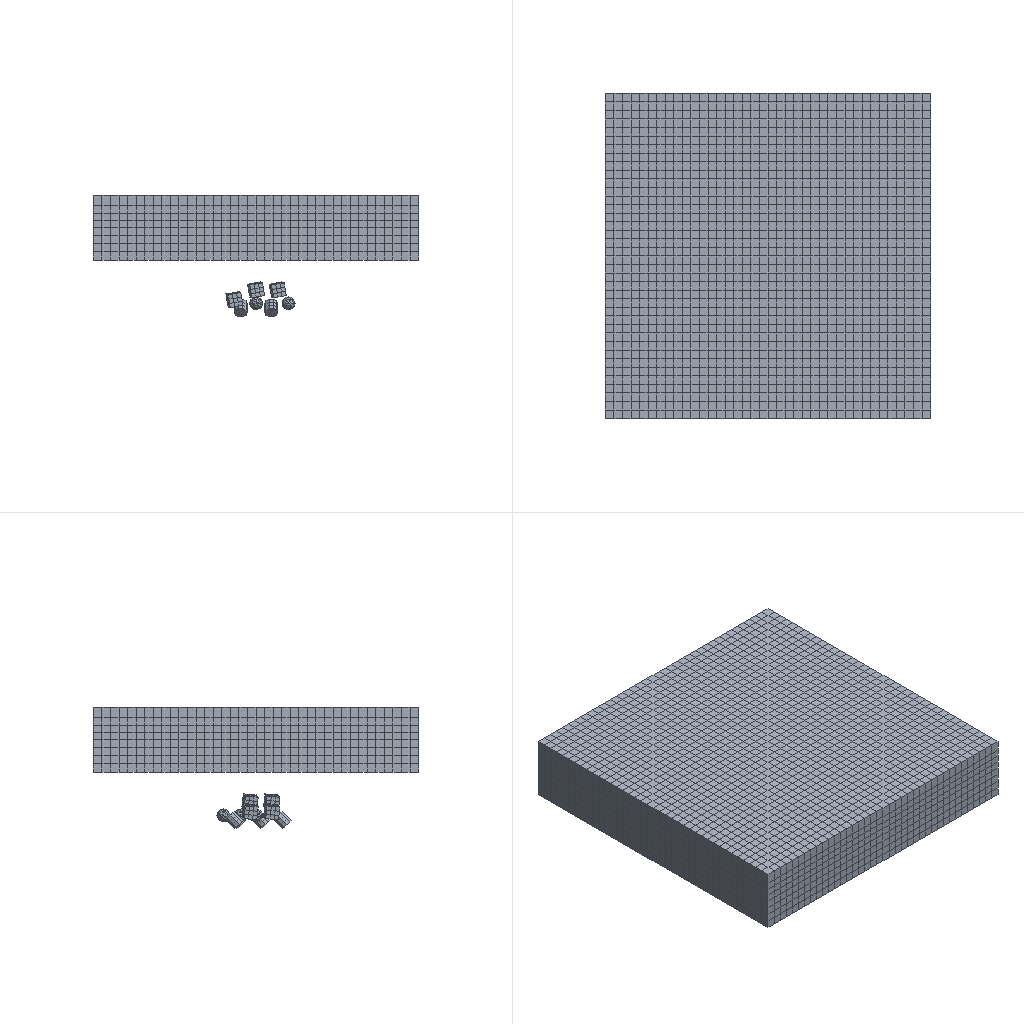Simulation study | abaqus
Set-up summary:
category,name,step,type,value,unit,region
solver,abaqus
solver,version,,,Abaqus/Standard 2020
units,not stated in the deck,,not stated
analysis,deck,,transient,transient
load_step,Step-1,Step-1,transient
load_step,requested,,,1
mesh,nodes,,,19847
mesh,elements,,,15155
element_type,C3D8R,,solid,11870
element_type,C3D10M,,solid,3285
load,load commands in deck,,count,1
bc,support commands in deck,,count,1
material,NIANTU,,in results
material,SHATU,,in results
material,SHI,,in results
material,YUNI,,in results
check,setup vs results,,match,"per instance, exact: element labels, types and connectivity; labels of the nodes the elements use; coordinates of those nodes at SINGLE_PRECISION in 15 of 16 instance(s)"
Abaqus input file, long lists of numbers shortened:
*Heading
** Job name: Job-2 Model name: Model-1-Copy
** Generated by: Abaqus/CAE 2020
*Preprint, echo=NO, model=NO, history=NO, contact=NO
**
** PARTS
**
*Part, name=base
*Node
      1,           0.,           0.,          1.5
      2,           0.,         -15.,          1.5
** (13687 more lines like these left out)
*Element, type=C3D8R
   1,  246,  925, 6845,  777,    1,   17,  629,   94
   2,  925,  926, 6846, 6845,   17,   18,  630,  629
** (11550 more lines like these left out)
*Nset, nset=Set-1
    3,    4,    6,    7,   13,   14,   15,   16,   56,   57,   58,   59,   60,   61,   62,   63
   64,   65,   66,   67,   68,   69,   70,   71,   72,   73,   74,   75,   76,   77,   78,   79
** (189 more lines like these left out)
*Elset, elset=Set-1, generate
 10109,  11552,      1
*Nset, nset=Set-2
    1,    2,    3,    4,    5,    6,    7,    8,   17,   18,   19,   20,   21,   22,   23,   24
   25,   26,   27,   28,   29,   30,   31,   32,   33,   34,   35,   36,   37,   38,   39,   40
** (379 more lines like these left out)
*Elset, elset=Set-2, generate
    1,  4332,     1
*Nset, nset=Set-3
     1,     2,     5,     8,     9,    10,    11,    12,    17,    18,    19,    20,    21,    22,    23,    24
    25,    26,    27,    28,    29,    30,    31,    32,    33,    34,    35,    36,    37,    38,    39,    40
** (474 more lines like these left out)
*Elset, elset=Set-3, generate
  4333,  10108,      1
** Section: niantu
*Solid Section, elset=Set-2, material=niantu
,
** Section: shatu
*Solid Section, elset=Set-3, material=shatu
,
** Section: yuni
*Solid Section, elset=Set-1, material=yuni
,
*End Part
**
*Part, name=fang
*Node
      1,           0., -0.6,  0.6
      2,           0., -0.4,  0.6
** (62 more lines like these left out)
*Element, type=C3D8R
 1, 17, 18, 22, 21,  1,  2,  6,  5
 2, 18, 19, 23, 22,  2,  3,  7,  6
** (25 more lines like these left out)
*Nset, nset=Set-1, generate
  1,  64,   1
*Elset, elset=Set-1, generate
  1,  27,   1
** Section: shi
*Solid Section, elset=Set-1, material=shi
,
*End Part
**
*Part, name=fangkuai
*Node
      1,  0.2427,           0.,  0.1763
      2, 0.09271,           0.,  0.2853
** (74 more lines like these left out)
*Element, type=C3D8R
 1,  6,  7,  8, 19, 25, 26, 27, 38
 2, 11, 14, 12, 19, 30, 33, 31, 38
** (37 more lines like these left out)
*Nset, nset=Set-1, generate
  1,  76,   1
*Elset, elset=Set-1, generate
  1,  39,   1
** Section: shi
*Solid Section, elset=Set-1, material=shi
,
*End Part
**
*Part, name=sphere
*Node
      1,  0.1148,  0.2772,           0.
      2,  0.2121,  0.2121,           0.
** (1092 more lines like these left out)
*Element, type=C3D10M
  1,  101,  102,  103,  104,  173,  172,  171,  175,  174,  176
  2,  105,  106,  102,  107,  179,  178,  177,  181,  180,  182
** (655 more lines like these left out)
*Nset, nset=Set-1, generate
    1,  1094,     1
*Elset, elset=Set-1, generate
   1,  657,    1
** Section: shi
*Solid Section, elset=Set-1, material=shi
,
*End Part
**
**
** ASSEMBLY
**
*Assembly, name=Assembly
**
*Instance, name=base-1, part=base
*End Instance
**
*Instance, name=sphere-1, part=sphere
         7.5,         -7.5,          -2.
*End Instance
**
*Instance, name=fangkuai-1, part=fangkuai
         8.2,         -7.5,          -2.
         8.2,         -7.5,          -2., 9.2,         -7.5,          -2., 45.
*End Instance
**
*Instance, name=fang-1, part=fang
6.209, -6.949, -2.154
6.209, -6.949, -2.154, 6.542, -7.616, -1.487, 15.
*End Instance
**
*Instance, name=sphere-1-lin-1-2, part=sphere
         7.5,         -6.8,          -2.
*End Instance
**
*Instance, name=sphere-1-lin-2-1, part=sphere
          9.,         -7.5,          -2.
*End Instance
**
*Instance, name=sphere-1-lin-2-2, part=sphere
          9.,         -6.8,          -2.
*End Instance
**
*Instance, name=fangkuai-1-lin-1-2, part=fangkuai
         8.2,         -6.4,          -2.
         8.2,         -6.4,          -2., 9.2,         -6.4,          -2., 45.
*End Instance
**
*Instance, name=fangkuai-1-lin-1-2-1, part=fangkuai
         8.2,         -8.5,          -2.
         8.2,         -8.5,          -2., 9.2,         -8.5,          -2., 45.
*End Instance
**
*Instance, name=fang-1-lin-1-2, part=fang
6.209, -7.949, -2.154
6.209, -7.949, -2.154, 6.542, -8.616, -1.487, 15.
*End Instance
**
*Instance, name=fang-1-lin-2-1, part=fang
7.209, -6.949, -1.704
7.209, -6.949, -1.704, 7.542, -7.616, -1.037, 15.
*End Instance
**
*Instance, name=fang-1-lin-2-2, part=fang
7.209, -7.949, -1.704
7.209, -7.949, -1.704, 7.542, -8.616, -1.037, 15.
*End Instance
**
*Instance, name=fang-1-lin-3-1, part=fang
8.209, -6.949, -1.704
8.209, -6.949, -1.704, 8.542, -7.616, -1.037, 15.
*End Instance
**
*Instance, name=fang-1-lin-3-2, part=fang
8.209, -7.949, -1.704
8.209, -7.949, -1.704, 8.542, -8.616, -1.037, 15.
*End Instance
**
*Instance, name=sphere-1-lin-1-2-lin-1-2, part=sphere
         7.5,          -6.,          -2.
*End Instance
**
*Instance, name=fangkuai-1-lin-1-2-lin-2-1, part=fangkuai
         6.8,         -6.3,          -2.
         6.8,         -6.3,          -2., 7.8,         -6.3,          -2., 45.
*End Instance
**
*Nset, nset=Set-1, instance=base-1
   13,   14,   15,   16,  481,  482,  483,  484,  485,  486,  487,  488,  489,  490,  491,  492
  493,  494,  495,  496,  497,  498,  499,  500,  501,  502,  503,  504,  505,  506,  507,  508
** (94 more lines like these left out)
*Elset, elset=Set-1, instance=base-1, generate
 10109,  11552,      1
*Nset, nset=Set-2, instance=sphere-1, generate
    1,  1094,     1
*Nset, nset=Set-2, instance=fangkuai-1, generate
  1,  76,   1
*Nset, nset=Set-2, instance=fang-1, generate
  1,  64,   1
*Nset, nset=Set-2, instance=fangkuai-1-lin-1-2, generate
  1,  76,   1
*Nset, nset=Set-2, instance=fangkuai-1-lin-1-2-lin-2-1, generate
  1,  76,   1
*Nset, nset=Set-2, instance=fang-1-lin-2-2, generate
  1,  64,   1
*Nset, nset=Set-2, instance=sphere-1-lin-2-1, generate
    1,  1094,     1
*Nset, nset=Set-2, instance=fang-1-lin-1-2, generate
  1,  64,   1
*Nset, nset=Set-2, instance=fang-1-lin-3-2, generate
  1,  64,   1
*Nset, nset=Set-2, instance=sphere-1-lin-1-2, generate
    1,  1094,     1
*Nset, nset=Set-2, instance=fangkuai-1-lin-1-2-1, generate
  1,  76,   1
*Nset, nset=Set-2, instance=fang-1-lin-3-1, generate
  1,  64,   1
*Nset, nset=Set-2, instance=sphere-1-lin-2-2, generate
    1,  1094,     1
*Nset, nset=Set-2, instance=fang-1-lin-2-1, generate
  1,  64,   1
*Nset, nset=Set-2, instance=sphere-1-lin-1-2-lin-1-2, generate
    1,  1094,     1
*Elset, elset=Set-2, instance=sphere-1, generate
   1,  657,    1
*Elset, elset=Set-2, instance=fangkuai-1, generate
  1,  39,   1
*Elset, elset=Set-2, instance=fang-1, generate
  1,  27,   1
*Elset, elset=Set-2, instance=fangkuai-1-lin-1-2, generate
  1,  39,   1
*Elset, elset=Set-2, instance=fangkuai-1-lin-1-2-lin-2-1, generate
  1,  39,   1
*Elset, elset=Set-2, instance=fang-1-lin-2-2, generate
  1,  27,   1
*Elset, elset=Set-2, instance=sphere-1-lin-2-1, generate
   1,  657,    1
*Elset, elset=Set-2, instance=fang-1-lin-1-2, generate
  1,  27,   1
*Elset, elset=Set-2, instance=fang-1-lin-3-2, generate
  1,  27,   1
*Elset, elset=Set-2, instance=sphere-1-lin-1-2, generate
   1,  657,    1
*Elset, elset=Set-2, instance=fangkuai-1-lin-1-2-1, generate
  1,  39,   1
*Elset, elset=Set-2, instance=fang-1-lin-3-1, generate
  1,  27,   1
*Elset, elset=Set-2, instance=sphere-1-lin-2-2, generate
   1,  657,    1
*Elset, elset=Set-2, instance=fang-1-lin-2-1, generate
  1,  27,   1
*Elset, elset=Set-2, instance=sphere-1-lin-1-2-lin-1-2, generate
   1,  657,    1
*Elset, elset=__Int-1_gcs0_17_S3, internal, instance=sphere-1
  37,  61,  70,  92, 110, 121, 137, 145, 146, 173, 197, 218, 224, 238, 277, 286
 298, 300, 327, 346, 399, 405, 411, 412, 414, 415, 421, 422, 425, 428, 434, 437
** (9 more lines like these left out)
*Elset, elset=__Int-1_gcs0_17_S4, internal, instance=sphere-1
  53,  84, 112, 166, 184, 251, 264, 265, 320, 624, 655
*Elset, elset=__Int-1_gcs0_17_S1, internal, instance=sphere-1
  67, 293, 381, 419
*Elset, elset=__Int-1_gcs0_17_S2, internal, instance=sphere-1
 220, 350, 409, 427, 447, 451, 588, 650
*Surface, type=ELEMENT, name=_Int-1_gcs0_17, internal
__Int-1_gcs0_17_S3, S3
__Int-1_gcs0_17_S4, S4
__Int-1_gcs0_17_S2, S2
__Int-1_gcs0_17_S1, S1
*Elset, elset=__Int-1_gcs0_18_S3, internal, instance=fangkuai-1
  1,  8, 14, 21, 27, 34
*Elset, elset=__Int-1_gcs0_18_S4, internal, instance=fangkuai-1
  1,  3,  4, 13, 14, 16, 17, 26, 27, 29, 30, 39
*Elset, elset=__Int-1_gcs0_18_S5, internal, instance=fangkuai-1
  5,  6, 11, 18, 19, 24, 31, 32, 37
*Elset, elset=__Int-1_gcs0_18_S6, internal, instance=fangkuai-1, generate
 10,  36,  13
*Surface, type=ELEMENT, name=_Int-1_gcs0_18, internal
__Int-1_gcs0_18_S3, S3
__Int-1_gcs0_18_S4, S4
__Int-1_gcs0_18_S6, S6
__Int-1_gcs0_18_S5, S5
*Elset, elset=__Int-1_gcs0_27_S3, internal, instance=sphere-1-lin-1-2
  37,  61,  70,  92, 110, 121, 137, 145, 146, 173, 197, 218, 224, 238, 277, 286
 298, 300, 327, 346, 399, 405, 411, 412, 414, 415, 421, 422, 425, 428, 434, 437
** (9 more lines like these left out)
*Elset, elset=__Int-1_gcs0_27_S4, internal, instance=sphere-1-lin-1-2
  53,  84, 112, 166, 184, 251, 264, 265, 320, 624, 655
*Elset, elset=__Int-1_gcs0_27_S1, internal, instance=sphere-1-lin-1-2
  67, 293, 381, 419
*Elset, elset=__Int-1_gcs0_27_S2, internal, instance=sphere-1-lin-1-2
 220, 350, 409, 427, 447, 451, 588, 650
*Surface, type=ELEMENT, name=_Int-1_gcs0_27, internal
__Int-1_gcs0_27_S3, S3
__Int-1_gcs0_27_S4, S4
__Int-1_gcs0_27_S2, S2
__Int-1_gcs0_27_S1, S1
*Elset, elset=__Int-1_gcs0_28_S3, internal, instance=sphere-1-lin-2-1
  37,  61,  70,  92, 110, 121, 137, 145, 146, 173, 197, 218, 224, 238, 277, 286
 298, 300, 327, 346, 399, 405, 411, 412, 414, 415, 421, 422, 425, 428, 434, 437
** (9 more lines like these left out)
*Elset, elset=__Int-1_gcs0_28_S4, internal, instance=sphere-1-lin-2-1
  53,  84, 112, 166, 184, 251, 264, 265, 320, 624, 655
*Elset, elset=__Int-1_gcs0_28_S1, internal, instance=sphere-1-lin-2-1
  67, 293, 381, 419
*Elset, elset=__Int-1_gcs0_28_S2, internal, instance=sphere-1-lin-2-1
 220, 350, 409, 427, 447, 451, 588, 650
*Surface, type=ELEMENT, name=_Int-1_gcs0_28, internal
__Int-1_gcs0_28_S3, S3
__Int-1_gcs0_28_S4, S4
__Int-1_gcs0_28_S2, S2
__Int-1_gcs0_28_S1, S1
*Elset, elset=__Int-1_gcs0_29_S3, internal, instance=sphere-1-lin-2-2
  37,  61,  70,  92, 110, 121, 137, 145, 146, 173, 197, 218, 224, 238, 277, 286
 298, 300, 327, 346, 399, 405, 411, 412, 414, 415, 421, 422, 425, 428, 434, 437
** (9 more lines like these left out)
*Elset, elset=__Int-1_gcs0_29_S4, internal, instance=sphere-1-lin-2-2
  53,  84, 112, 166, 184, 251, 264, 265, 320, 624, 655
*Elset, elset=__Int-1_gcs0_29_S1, internal, instance=sphere-1-lin-2-2
  67, 293, 381, 419
*Elset, elset=__Int-1_gcs0_29_S2, internal, instance=sphere-1-lin-2-2
 220, 350, 409, 427, 447, 451, 588, 650
*Surface, type=ELEMENT, name=_Int-1_gcs0_29, internal
__Int-1_gcs0_29_S3, S3
__Int-1_gcs0_29_S4, S4
__Int-1_gcs0_29_S2, S2
__Int-1_gcs0_29_S1, S1
*Elset, elset=__Int-1_gcs0_30_S3, internal, instance=fangkuai-1-lin-1-2
  1,  8, 14, 21, 27, 34
*Elset, elset=__Int-1_gcs0_30_S4, internal, instance=fangkuai-1-lin-1-2
  1,  3,  4, 13, 14, 16, 17, 26, 27, 29, 30, 39
*Elset, elset=__Int-1_gcs0_30_S5, internal, instance=fangkuai-1-lin-1-2
  5,  6, 11, 18, 19, 24, 31, 32, 37
*Elset, elset=__Int-1_gcs0_30_S6, internal, instance=fangkuai-1-lin-1-2, generate
 10,  36,  13
*Surface, type=ELEMENT, name=_Int-1_gcs0_30, internal
__Int-1_gcs0_30_S3, S3
__Int-1_gcs0_30_S4, S4
__Int-1_gcs0_30_S6, S6
__Int-1_gcs0_30_S5, S5
*Elset, elset=__Int-1_gcs0_33_S3, internal, instance=fangkuai-1-lin-1-2-1
  1,  8, 14, 21, 27, 34
*Elset, elset=__Int-1_gcs0_33_S4, internal, instance=fangkuai-1-lin-1-2-1
  1,  3,  4, 13, 14, 16, 17, 26, 27, 29, 30, 39
*Elset, elset=__Int-1_gcs0_33_S5, internal, instance=fangkuai-1-lin-1-2-1
  5,  6, 11, 18, 19, 24, 31, 32, 37
*Elset, elset=__Int-1_gcs0_33_S6, internal, instance=fangkuai-1-lin-1-2-1, generate
 10,  36,  13
*Surface, type=ELEMENT, name=_Int-1_gcs0_33, internal
__Int-1_gcs0_33_S3, S3
__Int-1_gcs0_33_S4, S4
__Int-1_gcs0_33_S6, S6
__Int-1_gcs0_33_S5, S5
*Elset, elset=__Int-1_gcs0_66_S3, internal, instance=sphere-1-lin-1-2-lin-1-2
  37,  61,  70,  92, 110, 121, 137, 145, 146, 173, 197, 218, 224, 238, 277, 286
 298, 300, 327, 346, 399, 405, 411, 412, 414, 415, 421, 422, 425, 428, 434, 437
** (9 more lines like these left out)
*Elset, elset=__Int-1_gcs0_66_S4, internal, instance=sphere-1-lin-1-2-lin-1-2
  53,  84, 112, 166, 184, 251, 264, 265, 320, 624, 655
*Elset, elset=__Int-1_gcs0_66_S1, internal, instance=sphere-1-lin-1-2-lin-1-2
  67, 293, 381, 419
*Elset, elset=__Int-1_gcs0_66_S2, internal, instance=sphere-1-lin-1-2-lin-1-2
 220, 350, 409, 427, 447, 451, 588, 650
*Surface, type=ELEMENT, name=_Int-1_gcs0_66, internal
__Int-1_gcs0_66_S3, S3
__Int-1_gcs0_66_S4, S4
__Int-1_gcs0_66_S2, S2
__Int-1_gcs0_66_S1, S1
*Elset, elset=__Int-1_gcs0_67_S3, internal, instance=fangkuai-1-lin-1-2-lin-2-1
  1,  8, 14, 21, 27, 34
*Elset, elset=__Int-1_gcs0_67_S4, internal, instance=fangkuai-1-lin-1-2-lin-2-1
  1,  3,  4, 13, 14, 16, 17, 26, 27, 29, 30, 39
*Elset, elset=__Int-1_gcs0_67_S5, internal, instance=fangkuai-1-lin-1-2-lin-2-1
  5,  6, 11, 18, 19, 24, 31, 32, 37
*Elset, elset=__Int-1_gcs0_67_S6, internal, instance=fangkuai-1-lin-1-2-lin-2-1, generate
 10,  36,  13
*Surface, type=ELEMENT, name=_Int-1_gcs0_67, internal
__Int-1_gcs0_67_S3, S3
__Int-1_gcs0_67_S4, S4
__Int-1_gcs0_67_S6, S6
__Int-1_gcs0_67_S5, S5
*End Assembly
**
** MATERIALS
**
*Material, name=niantu
*Density
1560.,
*Elastic
 6e+08, 0.35
*Material, name=shatu
*Density
2300.,
*Elastic
 2e+09, 0.36
*Material, name=shi
*Density
2850.,
*Elastic
 2e+10, 0.22
*Material, name=yuni
*Density
1200.,
*Elastic
 6e+09, 0.35
**
** INTERACTION PROPERTIES
**
*Surface Interaction, name=IntProp-1
1.,
*Friction, slip tolerance=0.005
 0.2,
*Surface Behavior, pressure-overclosure=HARD
**
** INTERACTIONS
**
** Interaction: Int-1
*Contact
*Contact Inclusions, ALL EXTERIOR
*Contact Property Assignment
 ,  , IntProp-1
*Surface Property Assignment, property=GEOMETRIC CORRECTION
_Int-1_gcs0_17, Spherical, 7.5, -7.5, -2.
_Int-1_gcs0_18, Circumferential, 8.2, -7.712, -2.212,  8.2, -8.419, -2.919
_Int-1_gcs0_27, Spherical, 7.5, -6.8, -2.
_Int-1_gcs0_28, Spherical, 9., -7.5, -2.
_Int-1_gcs0_29, Spherical, 9., -6.8, -2.
_Int-1_gcs0_30, Circumferential, 8.2, -6.612, -2.212,  8.2, -7.319, -2.919
_Int-1_gcs0_33, Circumferential, 8.2, -8.712, -2.212,  8.2, -9.419, -2.919
_Int-1_gcs0_66, Spherical, 7.5, -6., -2.
_Int-1_gcs0_67, Circumferential, 6.8, -6.512, -2.212,  6.8, -7.219, -2.919
** ----------------------------------------------------------------
**
** STEP: Step-1
**
*Step, name=Step-1, nlgeom=YES, inc=1000
*Dynamic
0.01,1.,1e-05
**
** BOUNDARY CONDITIONS
**
** Name: BC-1 Type: 对称/反对称/完全固定
*Boundary
Set-1, ENCASTRE
**
** LOADS
**
** Name: Load-1   Type: Gravity
*Dload
Set-2, GRAV, 9.8, 0., 0., 1.
**
** OUTPUT REQUESTS
**
*Restart, write, number interval=1, time marks=NO
**
** FIELD OUTPUT: F-Output-1
**
*Output, field, variable=PRESELECT, frequency=1
**
** HISTORY OUTPUT: H-Output-1
**
*Output, history, variable=PRESELECT, number interval=200, time marks=NO
*End Step
Results summary:
result,step,,completed,increments=163 time=1.0/1.0
result,analysis,,,transient
result,last_loadstep,,,1
result,primary field,,,U
result,reaction total,,FX,22531.997,model units
result,reaction total,,FY,40340.723,model units
result,reaction total,,FZ,-206906.512,model units